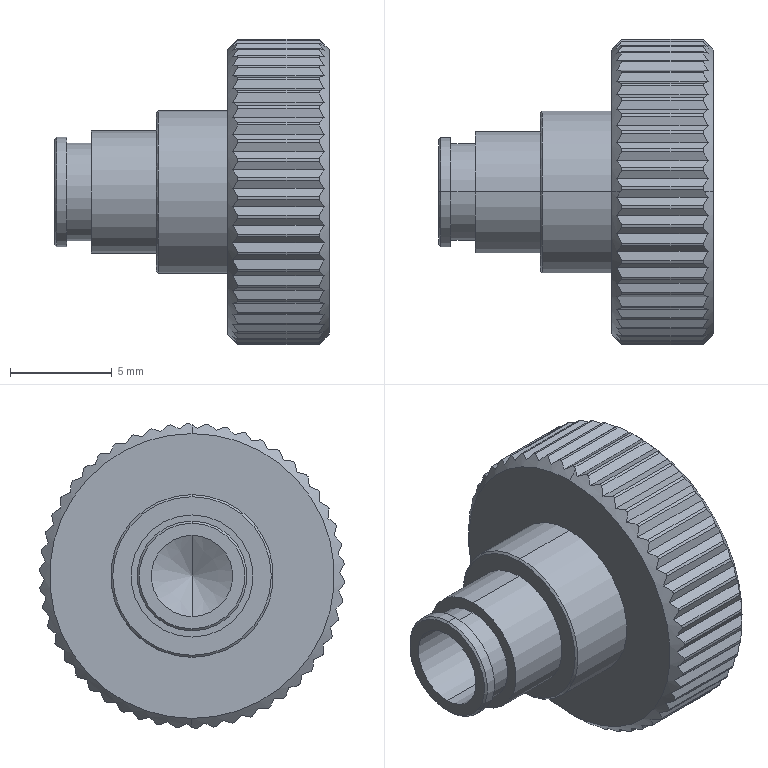Part | SolidWorks | features BaseBody 1 | 1 solid | 176 faces | box 13.5 x 14.994 x 14.998 mm | volume 1096 mm3 | plane 106 | cylinder 60 | cone 10 | commonest cylinder face diameters 15 x50 4 x2 4.8 x2 5.4 x2 6 x2 8 x2